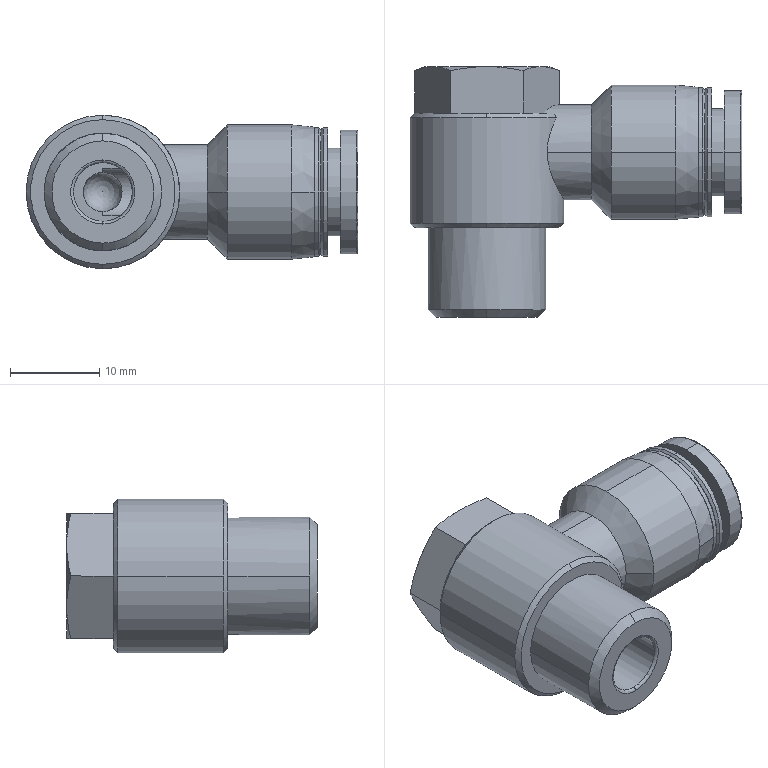Part | STEP file | PH802. | 1 solid | 74 faces | box 37.083 x 28 x 17.166 mm | volume 6341 mm3 | cylinder 23 | plane 23 | cone 21 | torus 6 | sphere 1 | commonest cylinder face diameters 14.4 x4 5.333 x2 6.579 x2 8 x2 9.8 x2 10.6 x2